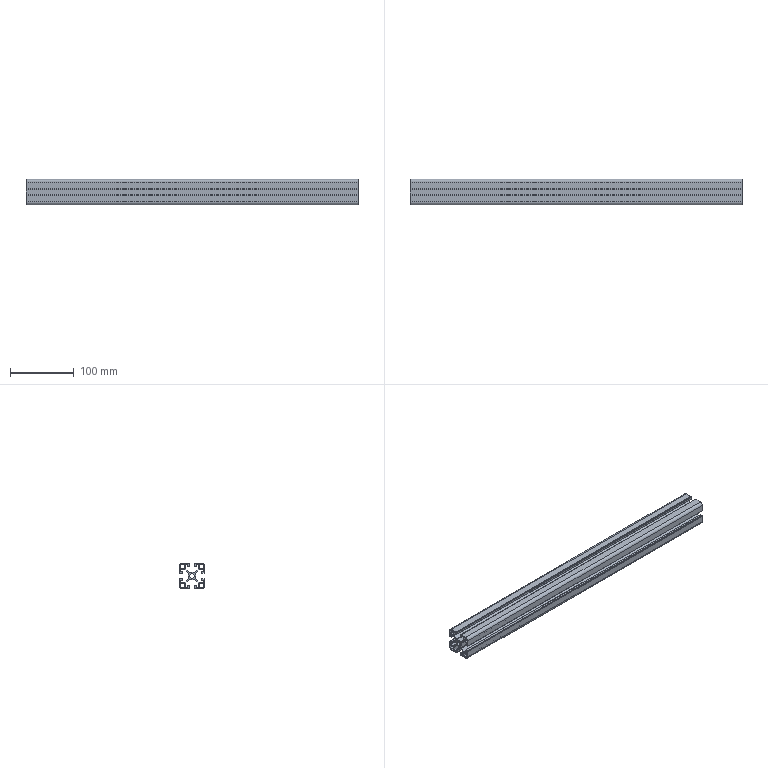Part | STEP file | Profile MK-8-4040C-L-00 4040C standard 520mm | 1 solid | 188 faces | box 520 x 40 x 40 mm | volume 248689 mm3 | cylinder 94 | plane 94 | commonest cylinder face diameters 0.6 x30 2 x28 4 x16 0.4 x8 6 x4 9 x4